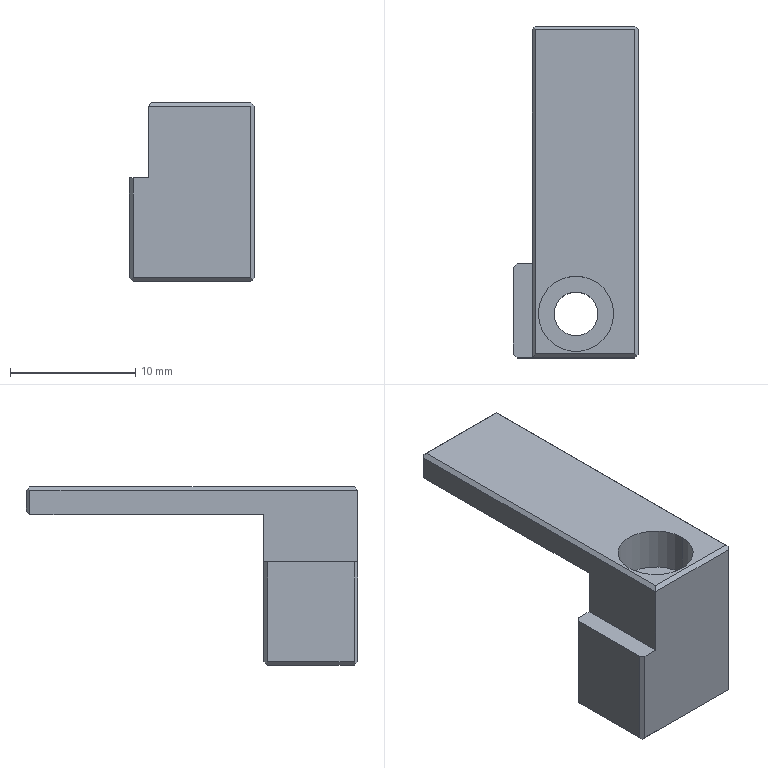Part | NX | 1 solid | 29 faces | box 10 x 26.45 x 14.25 mm | volume 1155 mm3 | plane 25 | cylinder 4 | commonest cylinder face diameters 3.5 x2 6 x2
STEP:
#1=CARTESIAN_POINT('',(-196.8,217.15,-49.35));
#2=VERTEX_POINT('',#1);
#3=CARTESIAN_POINT('',(-196.8,217.15,-47.4));
#4=VERTEX_POINT('',#3);
#5=CARTESIAN_POINT('',(-196.8,217.15,-48.375));
#6=DIRECTION('',(0.,0.,1.));
#7=VECTOR('',#6,1000.);
#8=LINE('',#5,#7);
#9=EDGE_CURVE('',#2,#4,#8,.T.);
#10=ORIENTED_EDGE('',*,*,#9,.T.);
#11=CARTESIAN_POINT('',(-196.8,191.3,-47.4));
#12=VERTEX_POINT('',#11);
#13=CARTESIAN_POINT('',(-196.8,212.,-47.4));
#14=DIRECTION('',(0.,-1.,0.));
#15=VECTOR('',#14,1000.);
#16=LINE('',#13,#15);
#17=EDGE_CURVE('',#4,#12,#16,.T.);
#18=ORIENTED_EDGE('',*,*,#17,.T.);
#19=CARTESIAN_POINT('',(-196.8,191.3,-61.05));
#20=VERTEX_POINT('',#19);
#21=CARTESIAN_POINT('',(-196.8,191.3,-54.225));
#22=DIRECTION('',(0.,0.,1.));
#23=VECTOR('',#22,1000.);
#24=LINE('',#21,#23);
#25=EDGE_CURVE('',#20,#12,#24,.T.);
#26=ORIENTED_EDGE('',*,*,#25,.F.);
#27=CARTESIAN_POINT('',(-196.8,198.5,-61.05));
#28=VERTEX_POINT('',#27);
#29=CARTESIAN_POINT('',(-196.8,194.75,-61.05));
#30=DIRECTION('',(0.,1.,0.));
#31=VECTOR('',#30,1000.);
#32=LINE('',#29,#31);
#33=EDGE_CURVE('',#20,#28,#32,.T.);
#34=ORIENTED_EDGE('',*,*,#33,.T.);
#35=CARTESIAN_POINT('',(-196.8,198.5,-49.35));
#36=VERTEX_POINT('',#35);
#37=CARTESIAN_POINT('',(-196.8,198.5,-40.731));
#38=DIRECTION('',(0.,0.,1.));
#39=VECTOR('',#38,1000.);
#40=LINE('',#37,#39);
#41=EDGE_CURVE('',#28,#36,#40,.T.);
#42=ORIENTED_EDGE('',*,*,#41,.T.);
#43=CARTESIAN_POINT('',(-196.8,212.,-49.35));
#44=DIRECTION('',(0.,-1.,0.));
#45=VECTOR('',#44,1000.);
#46=LINE('',#43,#45);
#47=EDGE_CURVE('',#2,#36,#46,.T.);
#48=ORIENTED_EDGE('',*,*,#47,.F.);
#49=EDGE_LOOP('',(#10,#18,#26,#34,#42,#48));
#50=FACE_BOUND('',#49,.T.);
#51=CARTESIAN_POINT('',(-196.8,212.,-46.1));
#52=DIRECTION('',(1.,0.,0.));
#53=DIRECTION('',(0.,1.,0.));
#54=AXIS2_PLACEMENT_3D('',#51,#52,#53);
#55=PLANE('',#54);
#56=ADVANCED_FACE('',(#50),#55,.T.);
#57=CARTESIAN_POINT('',(-197.1,217.15,-47.1));
#58=VERTEX_POINT('',#57);
#59=CARTESIAN_POINT('',(-205.,217.15,-47.1));
#60=VERTEX_POINT('',#59);
#61=CARTESIAN_POINT('',(-201.05,217.15,-47.1));
#62=DIRECTION('',(-1.,0.,0.));
#63=VECTOR('',#62,1000.);
#64=LINE('',#61,#63);
#65=EDGE_CURVE('',#58,#60,#64,.T.);
#66=ORIENTED_EDGE('',*,*,#65,.T.);
#67=CARTESIAN_POINT('',(-205.,191.3,-47.1));
#68=VERTEX_POINT('',#67);
#69=CARTESIAN_POINT('',(-205.,212.,-47.1));
#70=DIRECTION('',(0.,1.,0.));
#71=VECTOR('',#70,1000.);
#72=LINE('',#69,#71);
#73=EDGE_CURVE('',#68,#60,#72,.T.);
#74=ORIENTED_EDGE('',*,*,#73,.F.);
#75=CARTESIAN_POINT('',(-197.1,191.3,-47.1));
#76=VERTEX_POINT('',#75);
#77=CARTESIAN_POINT('',(-213.325,191.3,-47.1));
#78=DIRECTION('',(1.,0.,0.));
#79=VECTOR('',#78,1000.);
#80=LINE('',#77,#79);
#81=EDGE_CURVE('',#68,#76,#80,.T.);
#82=ORIENTED_EDGE('',*,*,#81,.T.);
#83=CARTESIAN_POINT('',(-197.1,212.,-47.1));
#84=DIRECTION('',(0.,-1.,0.));
#85=VECTOR('',#84,1000.);
#86=LINE('',#83,#85);
#87=EDGE_CURVE('',#58,#76,#86,.T.);
#88=ORIENTED_EDGE('',*,*,#87,.F.);
#89=EDGE_LOOP('',(#66,#74,#82,#88));
#90=FACE_BOUND('',#89,.T.);
#91=CARTESIAN_POINT('',(-198.8,194.5,-47.1));
#92=VERTEX_POINT('',#91);
#93=CARTESIAN_POINT('',(-204.8,194.5,-47.1));
#94=VERTEX_POINT('',#93);
#95=CARTESIAN_POINT('',(-201.8,194.5,-47.1));
#96=DIRECTION('',(0.,0.,1.));
#97=DIRECTION('',(-1.,0.,0.));
#98=AXIS2_PLACEMENT_3D('',#95,#96,#97);
#99=CIRCLE('',#98,3.);
#100=EDGE_CURVE('',#92,#94,#99,.T.);
#101=ORIENTED_EDGE('',*,*,#100,.F.);
#102=CARTESIAN_POINT('',(-201.8,194.5,-47.1));
#103=DIRECTION('',(0.,0.,1.));
#104=DIRECTION('',(-1.,0.,0.));
#105=AXIS2_PLACEMENT_3D('',#102,#103,#104);
#106=CIRCLE('',#105,3.);
#107=EDGE_CURVE('',#94,#92,#106,.T.);
#108=ORIENTED_EDGE('',*,*,#107,.F.);
#109=EDGE_LOOP('',(#101,#108));
#110=FACE_BOUND('',#109,.T.);
#111=CARTESIAN_POINT('',(-207.8,212.,-47.1));
#112=DIRECTION('',(0.,0.,1.));
#113=DIRECTION('',(0.,-1.,0.));
#114=AXIS2_PLACEMENT_3D('',#111,#112,#113);
#115=PLANE('',#114);
#116=ADVANCED_FACE('',(#90,#110),#115,.T.);
#117=CARTESIAN_POINT('',(-205.3,217.15,-49.35));
#118=VERTEX_POINT('',#117);
#119=CARTESIAN_POINT('',(-201.05,217.15,-49.35));
#120=DIRECTION('',(1.,0.,0.));
#121=VECTOR('',#120,1000.);
#122=LINE('',#119,#121);
#123=EDGE_CURVE('',#118,#2,#122,.T.);
#124=ORIENTED_EDGE('',*,*,#123,.T.);
#125=ORIENTED_EDGE('',*,*,#47,.T.);
#126=CARTESIAN_POINT('',(-205.3,198.5,-49.35));
#127=VERTEX_POINT('',#126);
#128=CARTESIAN_POINT('',(-213.325,198.5,-49.35));
#129=DIRECTION('',(1.,0.,0.));
#130=VECTOR('',#129,1000.);
#131=LINE('',#128,#130);
#132=EDGE_CURVE('',#127,#36,#131,.T.);
#133=ORIENTED_EDGE('',*,*,#132,.F.);
#134=CARTESIAN_POINT('',(-205.3,212.,-49.35));
#135=DIRECTION('',(0.,-1.,0.));
#136=VECTOR('',#135,1000.);
#137=LINE('',#134,#136);
#138=EDGE_CURVE('',#118,#127,#137,.T.);
#139=ORIENTED_EDGE('',*,*,#138,.F.);
#140=EDGE_LOOP('',(#124,#125,#133,#139));
#141=FACE_BOUND('',#140,.T.);
#142=CARTESIAN_POINT('',(-195.8,212.,-49.35));
#143=DIRECTION('',(0.,0.,-1.));
#144=DIRECTION('',(-1.,0.,0.));
#145=AXIS2_PLACEMENT_3D('',#142,#143,#144);
#146=PLANE('',#145);
#147=ADVANCED_FACE('',(#141),#146,.T.);
#148=CARTESIAN_POINT('',(-206.8,198.2,-53.1));
#149=VERTEX_POINT('',#148);
#150=CARTESIAN_POINT('',(-206.8,198.2,-61.05));
#151=VERTEX_POINT('',#150);
#152=CARTESIAN_POINT('',(-206.8,198.2,-57.225));
#153=DIRECTION('',(0.,0.,-1.));
#154=VECTOR('',#153,1000.);
#155=LINE('',#152,#154);
#156=EDGE_CURVE('',#149,#151,#155,.T.);
#157=ORIENTED_EDGE('',*,*,#156,.T.);
#158=CARTESIAN_POINT('',(-206.8,191.3,-61.05));
#159=VERTEX_POINT('',#158);
#160=CARTESIAN_POINT('',(-206.8,194.75,-61.05));
#161=DIRECTION('',(0.,-1.,0.));
#162=VECTOR('',#161,1000.);
#163=LINE('',#160,#162);
#164=EDGE_CURVE('',#151,#159,#163,.T.);
#165=ORIENTED_EDGE('',*,*,#164,.T.);
#166=CARTESIAN_POINT('',(-206.8,191.3,-53.1));
#167=VERTEX_POINT('',#166);
#168=CARTESIAN_POINT('',(-206.8,191.3,-57.225));
#169=DIRECTION('',(0.,0.,-1.));
#170=VECTOR('',#169,1000.);
#171=LINE('',#168,#170);
#172=EDGE_CURVE('',#167,#159,#171,.T.);
#173=ORIENTED_EDGE('',*,*,#172,.F.);
#174=CARTESIAN_POINT('',(-206.8,212.,-53.1));
#175=DIRECTION('',(0.,-1.,0.));
#176=VECTOR('',#175,1000.);
#177=LINE('',#174,#176);
#178=EDGE_CURVE('',#149,#167,#177,.T.);
#179=ORIENTED_EDGE('',*,*,#178,.F.);
#180=EDGE_LOOP('',(#157,#165,#173,#179));
#181=FACE_BOUND('',#180,.T.);
#182=CARTESIAN_POINT('',(-206.8,212.,-50.35));
#183=DIRECTION('',(-1.,0.,0.));
#184=DIRECTION('',(0.,1.,0.));
#185=AXIS2_PLACEMENT_3D('',#182,#183,#184);
#186=PLANE('',#185);
#187=ADVANCED_FACE('',(#181),#186,.T.);
#188=CARTESIAN_POINT('',(-197.1,191.3,-61.35));
#189=VERTEX_POINT('',#188);
#190=CARTESIAN_POINT('',(-197.1,198.2,-61.35));
#191=VERTEX_POINT('',#190);
#192=CARTESIAN_POINT('',(-197.1,194.75,-61.35));
#193=DIRECTION('',(0.,1.,0.));
#194=VECTOR('',#193,1000.);
#195=LINE('',#192,#194);
#196=EDGE_CURVE('',#189,#191,#195,.T.);
#197=ORIENTED_EDGE('',*,*,#196,.F.);
#198=CARTESIAN_POINT('',(-206.5,191.3,-61.35));
#199=VERTEX_POINT('',#198);
#200=CARTESIAN_POINT('',(-201.8,191.3,-61.35));
#201=DIRECTION('',(-1.,0.,0.));
#202=VECTOR('',#201,1000.);
#203=LINE('',#200,#202);
#204=EDGE_CURVE('',#189,#199,#203,.T.);
#205=ORIENTED_EDGE('',*,*,#204,.T.);
#206=CARTESIAN_POINT('',(-206.5,198.2,-61.35));
#207=VERTEX_POINT('',#206);
#208=CARTESIAN_POINT('',(-206.5,194.75,-61.35));
#209=DIRECTION('',(0.,-1.,0.));
#210=VECTOR('',#209,1000.);
#211=LINE('',#208,#210);
#212=EDGE_CURVE('',#207,#199,#211,.T.);
#213=ORIENTED_EDGE('',*,*,#212,.F.);
#214=CARTESIAN_POINT('',(-201.8,198.2,-61.35));
#215=DIRECTION('',(-1.,0.,0.));
#216=VECTOR('',#215,1000.);
#217=LINE('',#214,#216);
#218=EDGE_CURVE('',#191,#207,#217,.T.);
#219=ORIENTED_EDGE('',*,*,#218,.F.);
#220=EDGE_LOOP('',(#197,#205,#213,#219));
#221=FACE_BOUND('',#220,.T.);
#222=CARTESIAN_POINT('',(-200.05,194.5,-61.35));
#223=VERTEX_POINT('',#222);
#224=CARTESIAN_POINT('',(-203.55,194.5,-61.35));
#225=VERTEX_POINT('',#224);
#226=CARTESIAN_POINT('',(-201.8,194.5,-61.35));
#227=DIRECTION('',(0.,0.,1.));
#228=DIRECTION('',(-1.,0.,0.));
#229=AXIS2_PLACEMENT_3D('',#226,#227,#228);
#230=CIRCLE('',#229,1.75);
#231=EDGE_CURVE('',#223,#225,#230,.T.);
#232=ORIENTED_EDGE('',*,*,#231,.T.);
#233=CARTESIAN_POINT('',(-201.8,194.5,-61.35));
#234=DIRECTION('',(0.,0.,1.));
#235=DIRECTION('',(-1.,0.,0.));
#236=AXIS2_PLACEMENT_3D('',#233,#234,#235);
#237=CIRCLE('',#236,1.75);
#238=EDGE_CURVE('',#225,#223,#237,.T.);
#239=ORIENTED_EDGE('',*,*,#238,.T.);
#240=EDGE_LOOP('',(#232,#239));
#241=FACE_BOUND('',#240,.T.);
#242=CARTESIAN_POINT('',(-200.781,198.33,-61.35));
#243=DIRECTION('',(0.,0.,-1.));
#244=DIRECTION('',(-1.,0.,0.));
#245=AXIS2_PLACEMENT_3D('',#242,#243,#244);
#246=PLANE('',#245);
#247=ADVANCED_FACE('',(#221,#241),#246,.T.);
#248=ORIENTED_EDGE('',*,*,#100,.T.);
#249=CARTESIAN_POINT('',(-204.8,194.5,-50.6));
#250=VERTEX_POINT('',#249);
#251=CARTESIAN_POINT('',(-204.8,194.5,-47.1));
#252=DIRECTION('',(0.,0.,1.));
#253=VECTOR('',#252,1000.);
#254=LINE('',#251,#253);
#255=EDGE_CURVE('',#94,#250,#254,.F.);
#256=ORIENTED_EDGE('',*,*,#255,.T.);
#257=CARTESIAN_POINT('',(-198.8,194.5,-50.6));
#258=VERTEX_POINT('',#257);
#259=CARTESIAN_POINT('',(-201.8,194.5,-50.6));
#260=DIRECTION('',(0.,0.,1.));
#261=DIRECTION('',(-1.,0.,0.));
#262=AXIS2_PLACEMENT_3D('',#259,#260,#261);
#263=CIRCLE('',#262,3.);
#264=EDGE_CURVE('',#258,#250,#263,.T.);
#265=ORIENTED_EDGE('',*,*,#264,.F.);
#266=CARTESIAN_POINT('',(-198.8,194.5,-47.1));
#267=DIRECTION('',(0.,0.,1.));
#268=VECTOR('',#267,1000.);
#269=LINE('',#266,#268);
#270=EDGE_CURVE('',#92,#258,#269,.F.);
#271=ORIENTED_EDGE('',*,*,#270,.F.);
#272=EDGE_LOOP('',(#248,#256,#265,#271));
#273=FACE_BOUND('',#272,.T.);
#274=CARTESIAN_POINT('',(-201.8,194.5,-47.1));
#275=DIRECTION('',(0.,0.,1.));
#276=DIRECTION('',(-1.,0.,0.));
#277=AXIS2_PLACEMENT_3D('',#274,#275,#276);
#278=CYLINDRICAL_SURFACE('',#277,3.);
#279=ADVANCED_FACE('',(#273),#278,.F.);
#280=CARTESIAN_POINT('',(-200.05,194.5,-50.6));
#281=VERTEX_POINT('',#280);
#282=CARTESIAN_POINT('',(-203.55,194.5,-50.6));
#283=VERTEX_POINT('',#282);
#284=CARTESIAN_POINT('',(-201.8,194.5,-50.6));
#285=DIRECTION('',(0.,0.,1.));
#286=DIRECTION('',(-1.,0.,0.));
#287=AXIS2_PLACEMENT_3D('',#284,#285,#286);
#288=CIRCLE('',#287,1.75);
#289=EDGE_CURVE('',#281,#283,#288,.T.);
#290=ORIENTED_EDGE('',*,*,#289,.T.);
#291=CARTESIAN_POINT('',(-203.55,194.5,-47.1));
#292=DIRECTION('',(0.,0.,1.));
#293=VECTOR('',#292,1000.);
#294=LINE('',#291,#293);
#295=EDGE_CURVE('',#283,#225,#294,.F.);
#296=ORIENTED_EDGE('',*,*,#295,.T.);
#297=ORIENTED_EDGE('',*,*,#231,.F.);
#298=CARTESIAN_POINT('',(-200.05,194.5,-47.1));
#299=DIRECTION('',(0.,0.,1.));
#300=VECTOR('',#299,1000.);
#301=LINE('',#298,#300);
#302=EDGE_CURVE('',#281,#223,#301,.F.);
#303=ORIENTED_EDGE('',*,*,#302,.F.);
#304=EDGE_LOOP('',(#290,#296,#297,#303));
#305=FACE_BOUND('',#304,.T.);
#306=CARTESIAN_POINT('',(-201.8,194.5,-47.1));
#307=DIRECTION('',(0.,0.,1.));
#308=DIRECTION('',(-1.,0.,0.));
#309=AXIS2_PLACEMENT_3D('',#306,#307,#308);
#310=CYLINDRICAL_SURFACE('',#309,1.75);
#311=ADVANCED_FACE('',(#305),#310,.F.);
#312=ORIENTED_EDGE('',*,*,#264,.T.);
#313=CARTESIAN_POINT('',(-201.8,194.5,-50.6));
#314=DIRECTION('',(0.,0.,1.));
#315=DIRECTION('',(-1.,0.,0.));
#316=AXIS2_PLACEMENT_3D('',#313,#314,#315);
#317=CIRCLE('',#316,3.);
#318=EDGE_CURVE('',#250,#258,#317,.T.);
#319=ORIENTED_EDGE('',*,*,#318,.T.);
#320=EDGE_LOOP('',(#312,#319));
#321=FACE_BOUND('',#320,.T.);
#322=ORIENTED_EDGE('',*,*,#289,.F.);
#323=CARTESIAN_POINT('',(-201.8,194.5,-50.6));
#324=DIRECTION('',(0.,0.,1.));
#325=DIRECTION('',(-1.,0.,0.));
#326=AXIS2_PLACEMENT_3D('',#323,#324,#325);
#327=CIRCLE('',#326,1.75);
#328=EDGE_CURVE('',#283,#281,#327,.T.);
#329=ORIENTED_EDGE('',*,*,#328,.F.);
#330=EDGE_LOOP('',(#322,#329));
#331=FACE_BOUND('',#330,.T.);
#332=CARTESIAN_POINT('',(-201.8,194.5,-50.6));
#333=DIRECTION('',(0.,0.,1.));
#334=DIRECTION('',(0.,-1.,0.));
#335=AXIS2_PLACEMENT_3D('',#332,#333,#334);
#336=PLANE('',#335);
#337=ADVANCED_FACE('',(#321,#331),#336,.T.);
#338=CARTESIAN_POINT('',(-205.3,217.15,-47.4));
#339=VERTEX_POINT('',#338);
#340=CARTESIAN_POINT('',(-205.3,217.15,-48.375));
#341=DIRECTION('',(0.,0.,1.));
#342=VECTOR('',#341,1000.);
#343=LINE('',#340,#342);
#344=EDGE_CURVE('',#118,#339,#343,.T.);
#345=ORIENTED_EDGE('',*,*,#344,.F.);
#346=ORIENTED_EDGE('',*,*,#138,.T.);
#347=CARTESIAN_POINT('',(-205.3,198.5,-53.1));
#348=VERTEX_POINT('',#347);
#349=CARTESIAN_POINT('',(-205.3,198.5,-40.731));
#350=DIRECTION('',(0.,0.,-1.));
#351=VECTOR('',#350,1000.);
#352=LINE('',#349,#351);
#353=EDGE_CURVE('',#127,#348,#352,.T.);
#354=ORIENTED_EDGE('',*,*,#353,.T.);
#355=CARTESIAN_POINT('',(-205.3,191.,-53.1));
#356=VERTEX_POINT('',#355);
#357=CARTESIAN_POINT('',(-205.3,188.9,-53.1));
#358=DIRECTION('',(0.,1.,0.));
#359=VECTOR('',#358,1000.);
#360=LINE('',#357,#359);
#361=EDGE_CURVE('',#356,#348,#360,.T.);
#362=ORIENTED_EDGE('',*,*,#361,.F.);
#363=CARTESIAN_POINT('',(-205.3,191.,-47.4));
#364=VERTEX_POINT('',#363);
#365=CARTESIAN_POINT('',(-205.3,191.,-40.731));
#366=DIRECTION('',(0.,0.,-1.));
#367=VECTOR('',#366,1000.);
#368=LINE('',#365,#367);
#369=EDGE_CURVE('',#364,#356,#368,.T.);
#370=ORIENTED_EDGE('',*,*,#369,.F.);
#371=CARTESIAN_POINT('',(-205.3,212.,-47.4));
#372=DIRECTION('',(0.,1.,0.));
#373=VECTOR('',#372,1000.);
#374=LINE('',#371,#373);
#375=EDGE_CURVE('',#364,#339,#374,.T.);
#376=ORIENTED_EDGE('',*,*,#375,.T.);
#377=EDGE_LOOP('',(#345,#346,#354,#362,#370,#376));
#378=FACE_BOUND('',#377,.T.);
#379=CARTESIAN_POINT('',(-205.3,188.9,-53.1));
#380=DIRECTION('',(1.,0.,0.));
#381=DIRECTION('',(0.,1.,0.));
#382=AXIS2_PLACEMENT_3D('',#379,#380,#381);
#383=PLANE('',#382);
#384=ADVANCED_FACE('',(#378),#383,.F.);
#385=ORIENTED_EDGE('',*,*,#178,.T.);
#386=CARTESIAN_POINT('',(-206.5,191.,-53.1));
#387=VERTEX_POINT('',#386);
#388=CARTESIAN_POINT('',(-227.5,212.,-53.1));
#389=DIRECTION('',(0.7071,-0.7071,0.));
#390=VECTOR('',#389,1000.);
#391=LINE('',#388,#390);
#392=EDGE_CURVE('',#167,#387,#391,.T.);
#393=ORIENTED_EDGE('',*,*,#392,.T.);
#394=CARTESIAN_POINT('',(-213.325,191.,-53.1));
#395=DIRECTION('',(-1.,0.,0.));
#396=VECTOR('',#395,1000.);
#397=LINE('',#394,#396);
#398=EDGE_CURVE('',#356,#387,#397,.T.);
#399=ORIENTED_EDGE('',*,*,#398,.F.);
#400=ORIENTED_EDGE('',*,*,#361,.T.);
#401=CARTESIAN_POINT('',(-206.5,198.5,-53.1));
#402=VERTEX_POINT('',#401);
#403=CARTESIAN_POINT('',(-213.325,198.5,-53.1));
#404=DIRECTION('',(-1.,0.,0.));
#405=VECTOR('',#404,1000.);
#406=LINE('',#403,#405);
#407=EDGE_CURVE('',#348,#402,#406,.T.);
#408=ORIENTED_EDGE('',*,*,#407,.T.);
#409=CARTESIAN_POINT('',(-193.,212.,-53.1));
#410=DIRECTION('',(-0.7071,-0.7071,0.));
#411=VECTOR('',#410,1000.);
#412=LINE('',#409,#411);
#413=EDGE_CURVE('',#402,#149,#412,.T.);
#414=ORIENTED_EDGE('',*,*,#413,.T.);
#415=EDGE_LOOP('',(#385,#393,#399,#400,#408,#414));
#416=FACE_BOUND('',#415,.T.);
#417=CARTESIAN_POINT('',(-210.5,188.9,-53.1));
#418=DIRECTION('',(0.,0.,-1.));
#419=DIRECTION('',(-1.,0.,0.));
#420=AXIS2_PLACEMENT_3D('',#417,#418,#419);
#421=PLANE('',#420);
#422=ADVANCED_FACE('',(#416),#421,.F.);
#423=ORIENTED_EDGE('',*,*,#218,.T.);
#424=CARTESIAN_POINT('',(-206.65,198.35,-61.2));
#425=VERTEX_POINT('',#424);
#426=CARTESIAN_POINT('',(-220.3,212.,-47.55));
#427=DIRECTION('',(0.5774,-0.5774,-0.5774));
#428=VECTOR('',#427,1000.);
#429=LINE('',#426,#428);
#430=EDGE_CURVE('',#425,#207,#429,.T.);
#431=ORIENTED_EDGE('',*,*,#430,.F.);
#432=CARTESIAN_POINT('',(-206.5,198.5,-61.05));
#433=VERTEX_POINT('',#432);
#434=CARTESIAN_POINT('',(-186.181,218.819,-40.731));
#435=DIRECTION('',(-0.5774,-0.5774,-0.5774));
#436=VECTOR('',#435,1000.);
#437=LINE('',#434,#436);
#438=EDGE_CURVE('',#433,#425,#437,.T.);
#439=ORIENTED_EDGE('',*,*,#438,.F.);
#440=CARTESIAN_POINT('',(-201.8,198.5,-61.05));
#441=DIRECTION('',(-1.,0.,0.));
#442=VECTOR('',#441,1000.);
#443=LINE('',#440,#442);
#444=EDGE_CURVE('',#28,#433,#443,.T.);
#445=ORIENTED_EDGE('',*,*,#444,.F.);
#446=CARTESIAN_POINT('',(-183.3,212.,-47.55));
#447=DIRECTION('',(-0.5774,-0.5774,-0.5774));
#448=VECTOR('',#447,1000.);
#449=LINE('',#446,#448);
#450=EDGE_CURVE('',#28,#191,#449,.T.);
#451=ORIENTED_EDGE('',*,*,#450,.T.);
#452=EDGE_LOOP('',(#423,#431,#439,#445,#451));
#453=FACE_BOUND('',#452,.T.);
#454=CARTESIAN_POINT('',(-201.8,198.35,-61.2));
#455=DIRECTION('',(0.,-0.7071,0.7071));
#456=DIRECTION('',(-1.,0.,0.));
#457=AXIS2_PLACEMENT_3D('',#454,#455,#456);
#458=PLANE('',#457);
#459=ADVANCED_FACE('',(#453),#458,.F.);
#460=ORIENTED_EDGE('',*,*,#156,.F.);
#461=ORIENTED_EDGE('',*,*,#413,.F.);
#462=CARTESIAN_POINT('',(-206.5,198.5,-57.225));
#463=DIRECTION('',(0.,0.,-1.));
#464=VECTOR('',#463,1000.);
#465=LINE('',#462,#464);
#466=EDGE_CURVE('',#402,#433,#465,.T.);
#467=ORIENTED_EDGE('',*,*,#466,.T.);
#468=ORIENTED_EDGE('',*,*,#438,.T.);
#469=CARTESIAN_POINT('',(-193.,212.,-74.85));
#470=DIRECTION('',(-0.5774,-0.5774,0.5774));
#471=VECTOR('',#470,1000.);
#472=LINE('',#469,#471);
#473=EDGE_CURVE('',#425,#151,#472,.T.);
#474=ORIENTED_EDGE('',*,*,#473,.T.);
#475=EDGE_LOOP('',(#460,#461,#467,#468,#474));
#476=FACE_BOUND('',#475,.T.);
#477=CARTESIAN_POINT('',(-206.65,198.35,-57.225));
#478=DIRECTION('',(-0.7071,0.7071,0.));
#479=DIRECTION('',(0.,0.,1.));
#480=AXIS2_PLACEMENT_3D('',#477,#478,#479);
#481=PLANE('',#480);
#482=ADVANCED_FACE('',(#476),#481,.T.);
#483=ORIENTED_EDGE('',*,*,#196,.T.);
#484=ORIENTED_EDGE('',*,*,#450,.F.);
#485=ORIENTED_EDGE('',*,*,#33,.F.);
#486=CARTESIAN_POINT('',(-196.95,191.15,-61.2));
#487=VERTEX_POINT('',#486);
#488=CARTESIAN_POINT('',(-176.1,212.,-40.35));
#489=DIRECTION('',(-0.5774,-0.5774,-0.5774));
#490=VECTOR('',#489,1000.);
#491=LINE('',#488,#490);
#492=EDGE_CURVE('',#20,#487,#491,.T.);
#493=ORIENTED_EDGE('',*,*,#492,.T.);
#494=CARTESIAN_POINT('',(-217.8,212.,-82.05));
#495=DIRECTION('',(-0.5774,0.5774,-0.5774));
#496=VECTOR('',#495,1000.);
#497=LINE('',#494,#496);
#498=EDGE_CURVE('',#487,#189,#497,.T.);
#499=ORIENTED_EDGE('',*,*,#498,.T.);
#500=EDGE_LOOP('',(#483,#484,#485,#493,#499));
#501=FACE_BOUND('',#500,.T.);
#502=CARTESIAN_POINT('',(-196.95,194.75,-61.2));
#503=DIRECTION('',(-0.7071,0.,0.7071));
#504=DIRECTION('',(0.,1.,0.));
#505=AXIS2_PLACEMENT_3D('',#502,#503,#504);
#506=PLANE('',#505);
#507=ADVANCED_FACE('',(#501),#506,.F.);
#508=ORIENTED_EDGE('',*,*,#204,.F.);
#509=ORIENTED_EDGE('',*,*,#498,.F.);
#510=CARTESIAN_POINT('',(-197.1,191.,-61.05));
#511=VERTEX_POINT('',#510);
#512=CARTESIAN_POINT('',(-176.1,212.,-82.05));
#513=DIRECTION('',(0.5774,0.5774,-0.5774));
#514=VECTOR('',#513,1000.);
#515=LINE('',#512,#514);
#516=EDGE_CURVE('',#511,#487,#515,.T.);
#517=ORIENTED_EDGE('',*,*,#516,.F.);
#518=CARTESIAN_POINT('',(-206.5,191.,-61.05));
#519=VERTEX_POINT('',#518);
#520=CARTESIAN_POINT('',(-201.8,191.,-61.05));
#521=DIRECTION('',(-1.,0.,0.));
#522=VECTOR('',#521,1000.);
#523=LINE('',#520,#522);
#524=EDGE_CURVE('',#511,#519,#523,.T.);
#525=ORIENTED_EDGE('',*,*,#524,.T.);
#526=CARTESIAN_POINT('',(-206.65,191.15,-61.2));
#527=VERTEX_POINT('',#526);
#528=CARTESIAN_POINT('',(-227.5,212.,-82.05));
#529=DIRECTION('',(0.5774,-0.5774,0.5774));
#530=VECTOR('',#529,1000.);
#531=LINE('',#528,#530);
#532=EDGE_CURVE('',#527,#519,#531,.T.);
#533=ORIENTED_EDGE('',*,*,#532,.F.);
#534=CARTESIAN_POINT('',(-185.8,212.,-82.05));
#535=DIRECTION('',(-0.5774,-0.5774,0.5774));
#536=VECTOR('',#535,1000.);
#537=LINE('',#534,#536);
#538=EDGE_CURVE('',#199,#527,#537,.T.);
#539=ORIENTED_EDGE('',*,*,#538,.F.);
#540=EDGE_LOOP('',(#508,#509,#517,#525,#533,#539));
#541=FACE_BOUND('',#540,.T.);
#542=CARTESIAN_POINT('',(-201.8,191.15,-61.2));
#543=DIRECTION('',(0.,-0.7071,-0.7071));
#544=DIRECTION('',(0.,-0.7071,0.7071));
#545=AXIS2_PLACEMENT_3D('',#542,#543,#544);
#546=PLANE('',#545);
#547=ADVANCED_FACE('',(#541),#546,.T.);
#548=ORIENTED_EDGE('',*,*,#212,.T.);
#549=ORIENTED_EDGE('',*,*,#538,.T.);
#550=CARTESIAN_POINT('',(-227.5,212.,-40.35));
#551=DIRECTION('',(-0.5774,0.5774,0.5774));
#552=VECTOR('',#551,1000.);
#553=LINE('',#550,#552);
#554=EDGE_CURVE('',#527,#159,#553,.T.);
#555=ORIENTED_EDGE('',*,*,#554,.T.);
#556=ORIENTED_EDGE('',*,*,#164,.F.);
#557=ORIENTED_EDGE('',*,*,#473,.F.);
#558=ORIENTED_EDGE('',*,*,#430,.T.);
#559=EDGE_LOOP('',(#548,#549,#555,#556,#557,#558));
#560=FACE_BOUND('',#559,.T.);
#561=CARTESIAN_POINT('',(-206.65,194.75,-61.2));
#562=DIRECTION('',(0.7071,0.,0.7071));
#563=DIRECTION('',(0.,-1.,0.));
#564=AXIS2_PLACEMENT_3D('',#561,#562,#563);
#565=PLANE('',#564);
#566=ADVANCED_FACE('',(#560),#565,.F.);
#567=ORIENTED_EDGE('',*,*,#17,.F.);
#568=CARTESIAN_POINT('',(-196.95,217.3,-47.25));
#569=VERTEX_POINT('',#568);
#570=CARTESIAN_POINT('',(-213.325,233.675,-30.875));
#571=DIRECTION('',(0.5774,-0.5774,-0.5774));
#572=VECTOR('',#571,1000.);
#573=LINE('',#570,#572);
#574=EDGE_CURVE('',#569,#4,#573,.T.);
#575=ORIENTED_EDGE('',*,*,#574,.F.);
#576=CARTESIAN_POINT('',(-213.325,200.925,-30.875));
#577=DIRECTION('',(0.5774,0.5774,-0.5774));
#578=VECTOR('',#577,1000.);
#579=LINE('',#576,#578);
#580=EDGE_CURVE('',#58,#569,#579,.T.);
#581=ORIENTED_EDGE('',*,*,#580,.F.);
#582=ORIENTED_EDGE('',*,*,#87,.T.);
#583=CARTESIAN_POINT('',(-196.95,191.15,-47.25));
#584=VERTEX_POINT('',#583);
#585=CARTESIAN_POINT('',(-217.8,212.,-26.4));
#586=DIRECTION('',(-0.5774,0.5774,0.5774));
#587=VECTOR('',#586,1000.);
#588=LINE('',#585,#587);
#589=EDGE_CURVE('',#584,#76,#588,.T.);
#590=ORIENTED_EDGE('',*,*,#589,.F.);
#591=CARTESIAN_POINT('',(-176.1,212.,-68.1));
#592=DIRECTION('',(0.5774,0.5774,-0.5774));
#593=VECTOR('',#592,1000.);
#594=LINE('',#591,#593);
#595=EDGE_CURVE('',#584,#12,#594,.T.);
#596=ORIENTED_EDGE('',*,*,#595,.T.);
#597=EDGE_LOOP('',(#567,#575,#581,#582,#590,#596));
#598=FACE_BOUND('',#597,.T.);
#599=CARTESIAN_POINT('',(-196.95,200.775,-47.25));
#600=DIRECTION('',(0.7071,0.,0.7071));
#601=DIRECTION('',(0.,-1.,0.));
#602=AXIS2_PLACEMENT_3D('',#599,#600,#601);
#603=PLANE('',#602);
#604=ADVANCED_FACE('',(#598),#603,.T.);
#605=ORIENTED_EDGE('',*,*,#375,.F.);
#606=CARTESIAN_POINT('',(-184.3,212.,-26.4));
#607=DIRECTION('',(0.5774,0.5774,0.5774));
#608=VECTOR('',#607,1000.);
#609=LINE('',#606,#608);
#610=EDGE_CURVE('',#364,#68,#609,.T.);
#611=ORIENTED_EDGE('',*,*,#610,.T.);
#612=ORIENTED_EDGE('',*,*,#73,.T.);
#613=CARTESIAN_POINT('',(-205.15,217.3,-47.25));
#614=VERTEX_POINT('',#613);
#615=CARTESIAN_POINT('',(-213.325,225.475,-55.425));
#616=DIRECTION('',(-0.5774,0.5774,-0.5774));
#617=VECTOR('',#616,1000.);
#618=LINE('',#615,#617);
#619=EDGE_CURVE('',#60,#614,#618,.T.);
#620=ORIENTED_EDGE('',*,*,#619,.T.);
#621=CARTESIAN_POINT('',(-210.45,212.,-52.55));
#622=DIRECTION('',(0.5774,0.5774,0.5774));
#623=VECTOR('',#622,1000.);
#624=LINE('',#621,#623);
#625=EDGE_CURVE('',#339,#614,#624,.T.);
#626=ORIENTED_EDGE('',*,*,#625,.F.);
#627=EDGE_LOOP('',(#605,#611,#612,#620,#626));
#628=FACE_BOUND('',#627,.T.);
#629=CARTESIAN_POINT('',(-205.15,200.775,-47.25));
#630=DIRECTION('',(0.7071,0.,-0.7071));
#631=DIRECTION('',(0.,-1.,0.));
#632=AXIS2_PLACEMENT_3D('',#629,#630,#631);
#633=PLANE('',#632);
#634=ADVANCED_FACE('',(#628),#633,.F.);
#635=ORIENTED_EDGE('',*,*,#65,.F.);
#636=ORIENTED_EDGE('',*,*,#580,.T.);
#637=CARTESIAN_POINT('',(-197.1,217.45,-47.4));
#638=VERTEX_POINT('',#637);
#639=CARTESIAN_POINT('',(-213.325,233.675,-63.625));
#640=DIRECTION('',(0.5774,-0.5774,0.5774));
#641=VECTOR('',#640,1000.);
#642=LINE('',#639,#641);
#643=EDGE_CURVE('',#638,#569,#642,.T.);
#644=ORIENTED_EDGE('',*,*,#643,.F.);
#645=CARTESIAN_POINT('',(-205.,217.45,-47.4));
#646=VERTEX_POINT('',#645);
#647=CARTESIAN_POINT('',(-201.05,217.45,-47.4));
#648=DIRECTION('',(-1.,0.,0.));
#649=VECTOR('',#648,1000.);
#650=LINE('',#647,#649);
#651=EDGE_CURVE('',#638,#646,#650,.T.);
#652=ORIENTED_EDGE('',*,*,#651,.T.);
#653=CARTESIAN_POINT('',(-210.45,212.,-41.95));
#654=DIRECTION('',(-0.5774,-0.5774,0.5774));
#655=VECTOR('',#654,1000.);
#656=LINE('',#653,#655);
#657=EDGE_CURVE('',#646,#614,#656,.T.);
#658=ORIENTED_EDGE('',*,*,#657,.T.);
#659=ORIENTED_EDGE('',*,*,#619,.F.);
#660=EDGE_LOOP('',(#635,#636,#644,#652,#658,#659));
#661=FACE_BOUND('',#660,.T.);
#662=CARTESIAN_POINT('',(-201.05,217.3,-47.25));
#663=DIRECTION('',(0.,0.7071,0.7071));
#664=DIRECTION('',(1.,0.,0.));
#665=AXIS2_PLACEMENT_3D('',#662,#663,#664);
#666=PLANE('',#665);
#667=ADVANCED_FACE('',(#661),#666,.T.);
#668=ORIENTED_EDGE('',*,*,#9,.F.);
#669=CARTESIAN_POINT('',(-197.1,217.45,-49.05));
#670=VERTEX_POINT('',#669);
#671=CARTESIAN_POINT('',(-205.419,225.769,-40.731));
#672=DIRECTION('',(0.5774,-0.5774,-0.5774));
#673=VECTOR('',#672,1000.);
#674=LINE('',#671,#673);
#675=EDGE_CURVE('',#670,#2,#674,.T.);
#676=ORIENTED_EDGE('',*,*,#675,.F.);
#677=CARTESIAN_POINT('',(-197.1,217.45,-48.375));
#678=DIRECTION('',(0.,0.,1.));
#679=VECTOR('',#678,1000.);
#680=LINE('',#677,#679);
#681=EDGE_CURVE('',#670,#638,#680,.T.);
#682=ORIENTED_EDGE('',*,*,#681,.T.);
#683=ORIENTED_EDGE('',*,*,#643,.T.);
#684=ORIENTED_EDGE('',*,*,#574,.T.);
#685=EDGE_LOOP('',(#668,#676,#682,#683,#684));
#686=FACE_BOUND('',#685,.T.);
#687=CARTESIAN_POINT('',(-196.95,217.3,-48.375));
#688=DIRECTION('',(0.7071,0.7071,0.));
#689=DIRECTION('',(0.,0.,-1.));
#690=AXIS2_PLACEMENT_3D('',#687,#688,#689);
#691=PLANE('',#690);
#692=ADVANCED_FACE('',(#686),#691,.T.);
#693=ORIENTED_EDGE('',*,*,#344,.T.);
#694=ORIENTED_EDGE('',*,*,#625,.T.);
#695=ORIENTED_EDGE('',*,*,#657,.F.);
#696=CARTESIAN_POINT('',(-205.,217.45,-49.05));
#697=VERTEX_POINT('',#696);
#698=CARTESIAN_POINT('',(-205.,217.45,-48.375));
#699=DIRECTION('',(0.,0.,1.));
#700=VECTOR('',#699,1000.);
#701=LINE('',#698,#700);
#702=EDGE_CURVE('',#697,#646,#701,.T.);
#703=ORIENTED_EDGE('',*,*,#702,.F.);
#704=CARTESIAN_POINT('',(-196.681,225.769,-40.731));
#705=DIRECTION('',(0.5774,0.5774,0.5774));
#706=VECTOR('',#705,1000.);
#707=LINE('',#704,#706);
#708=EDGE_CURVE('',#118,#697,#707,.T.);
#709=ORIENTED_EDGE('',*,*,#708,.F.);
#710=EDGE_LOOP('',(#693,#694,#695,#703,#709));
#711=FACE_BOUND('',#710,.T.);
#712=CARTESIAN_POINT('',(-205.15,217.3,-48.375));
#713=DIRECTION('',(0.7071,-0.7071,0.));
#714=DIRECTION('',(0.,0.,-1.));
#715=AXIS2_PLACEMENT_3D('',#712,#713,#714);
#716=PLANE('',#715);
#717=ADVANCED_FACE('',(#711),#716,.F.);
#718=ORIENTED_EDGE('',*,*,#255,.F.);
#719=ORIENTED_EDGE('',*,*,#107,.T.);
#720=ORIENTED_EDGE('',*,*,#270,.T.);
#721=ORIENTED_EDGE('',*,*,#318,.F.);
#722=EDGE_LOOP('',(#718,#719,#720,#721));
#723=FACE_BOUND('',#722,.T.);
#724=CARTESIAN_POINT('',(-201.8,194.5,-47.1));
#725=DIRECTION('',(0.,0.,1.));
#726=DIRECTION('',(-1.,0.,0.));
#727=AXIS2_PLACEMENT_3D('',#724,#725,#726);
#728=CYLINDRICAL_SURFACE('',#727,3.);
#729=ADVANCED_FACE('',(#723),#728,.F.);
#730=ORIENTED_EDGE('',*,*,#295,.F.);
#731=ORIENTED_EDGE('',*,*,#328,.T.);
#732=ORIENTED_EDGE('',*,*,#302,.T.);
#733=ORIENTED_EDGE('',*,*,#238,.F.);
#734=EDGE_LOOP('',(#730,#731,#732,#733));
#735=FACE_BOUND('',#734,.T.);
#736=CARTESIAN_POINT('',(-201.8,194.5,-47.1));
#737=DIRECTION('',(0.,0.,1.));
#738=DIRECTION('',(-1.,0.,0.));
#739=AXIS2_PLACEMENT_3D('',#736,#737,#738);
#740=CYLINDRICAL_SURFACE('',#739,1.75);
#741=ADVANCED_FACE('',(#735),#740,.F.);
#742=CARTESIAN_POINT('',(-206.5,191.,-57.225));
#743=DIRECTION('',(0.,0.,-1.));
#744=VECTOR('',#743,1000.);
#745=LINE('',#742,#744);
#746=EDGE_CURVE('',#387,#519,#745,.T.);
#747=ORIENTED_EDGE('',*,*,#746,.T.);
#748=ORIENTED_EDGE('',*,*,#524,.F.);
#749=CARTESIAN_POINT('',(-197.1,191.,-47.4));
#750=VERTEX_POINT('',#749);
#751=CARTESIAN_POINT('',(-197.1,191.,-54.225));
#752=DIRECTION('',(0.,0.,1.));
#753=VECTOR('',#752,1000.);
#754=LINE('',#751,#753);
#755=EDGE_CURVE('',#511,#750,#754,.T.);
#756=ORIENTED_EDGE('',*,*,#755,.T.);
#757=CARTESIAN_POINT('',(-201.05,191.,-47.4));
#758=DIRECTION('',(1.,0.,0.));
#759=VECTOR('',#758,1000.);
#760=LINE('',#757,#759);
#761=EDGE_CURVE('',#364,#750,#760,.T.);
#762=ORIENTED_EDGE('',*,*,#761,.F.);
#763=ORIENTED_EDGE('',*,*,#369,.T.);
#764=ORIENTED_EDGE('',*,*,#398,.T.);
#765=EDGE_LOOP('',(#747,#748,#756,#762,#763,#764));
#766=FACE_BOUND('',#765,.T.);
#767=CARTESIAN_POINT('',(-213.325,191.,-40.731));
#768=DIRECTION('',(0.,1.,0.));
#769=DIRECTION('',(0.,0.,-1.));
#770=AXIS2_PLACEMENT_3D('',#767,#768,#769);
#771=PLANE('',#770);
#772=ADVANCED_FACE('',(#766),#771,.F.);
#773=ORIENTED_EDGE('',*,*,#610,.F.);
#774=ORIENTED_EDGE('',*,*,#761,.T.);
#775=CARTESIAN_POINT('',(-176.1,212.,-26.4));
#776=DIRECTION('',(-0.5774,-0.5774,-0.5774));
#777=VECTOR('',#776,1000.);
#778=LINE('',#775,#777);
#779=EDGE_CURVE('',#584,#750,#778,.T.);
#780=ORIENTED_EDGE('',*,*,#779,.F.);
#781=ORIENTED_EDGE('',*,*,#589,.T.);
#782=ORIENTED_EDGE('',*,*,#81,.F.);
#783=EDGE_LOOP('',(#773,#774,#780,#781,#782));
#784=FACE_BOUND('',#783,.T.);
#785=CARTESIAN_POINT('',(-201.05,191.15,-47.25));
#786=DIRECTION('',(0.,0.7071,-0.7071));
#787=DIRECTION('',(-1.,0.,0.));
#788=AXIS2_PLACEMENT_3D('',#785,#786,#787);
#789=PLANE('',#788);
#790=ADVANCED_FACE('',(#784),#789,.F.);
#791=ORIENTED_EDGE('',*,*,#755,.F.);
#792=ORIENTED_EDGE('',*,*,#516,.T.);
#793=ORIENTED_EDGE('',*,*,#492,.F.);
#794=ORIENTED_EDGE('',*,*,#25,.T.);
#795=ORIENTED_EDGE('',*,*,#595,.F.);
#796=ORIENTED_EDGE('',*,*,#779,.T.);
#797=EDGE_LOOP('',(#791,#792,#793,#794,#795,#796));
#798=FACE_BOUND('',#797,.T.);
#799=CARTESIAN_POINT('',(-196.95,191.15,-54.225));
#800=DIRECTION('',(0.7071,-0.7071,0.));
#801=DIRECTION('',(0.,0.,-1.));
#802=AXIS2_PLACEMENT_3D('',#799,#800,#801);
#803=PLANE('',#802);
#804=ADVANCED_FACE('',(#798),#803,.T.);
#805=ORIENTED_EDGE('',*,*,#746,.F.);
#806=ORIENTED_EDGE('',*,*,#392,.F.);
#807=ORIENTED_EDGE('',*,*,#172,.T.);
#808=ORIENTED_EDGE('',*,*,#554,.F.);
#809=ORIENTED_EDGE('',*,*,#532,.T.);
#810=EDGE_LOOP('',(#805,#806,#807,#808,#809));
#811=FACE_BOUND('',#810,.T.);
#812=CARTESIAN_POINT('',(-206.65,191.15,-57.225));
#813=DIRECTION('',(-0.7071,-0.7071,0.));
#814=DIRECTION('',(-0.7071,0.7071,0.));
#815=AXIS2_PLACEMENT_3D('',#812,#813,#814);
#816=PLANE('',#815);
#817=ADVANCED_FACE('',(#811),#816,.T.);
#818=CARTESIAN_POINT('',(-201.05,217.45,-49.05));
#819=DIRECTION('',(1.,0.,0.));
#820=VECTOR('',#819,1000.);
#821=LINE('',#818,#820);
#822=EDGE_CURVE('',#697,#670,#821,.T.);
#823=ORIENTED_EDGE('',*,*,#822,.F.);
#824=ORIENTED_EDGE('',*,*,#702,.T.);
#825=ORIENTED_EDGE('',*,*,#651,.F.);
#826=ORIENTED_EDGE('',*,*,#681,.F.);
#827=EDGE_LOOP('',(#823,#824,#825,#826));
#828=FACE_BOUND('',#827,.T.);
#829=CARTESIAN_POINT('',(-213.325,217.45,-40.731));
#830=DIRECTION('',(0.,1.,0.));
#831=DIRECTION('',(0.,0.,-1.));
#832=AXIS2_PLACEMENT_3D('',#829,#830,#831);
#833=PLANE('',#832);
#834=ADVANCED_FACE('',(#828),#833,.T.);
#835=ORIENTED_EDGE('',*,*,#132,.T.);
#836=ORIENTED_EDGE('',*,*,#41,.F.);
#837=ORIENTED_EDGE('',*,*,#444,.T.);
#838=ORIENTED_EDGE('',*,*,#466,.F.);
#839=ORIENTED_EDGE('',*,*,#407,.F.);
#840=ORIENTED_EDGE('',*,*,#353,.F.);
#841=EDGE_LOOP('',(#835,#836,#837,#838,#839,#840));
#842=FACE_BOUND('',#841,.T.);
#843=CARTESIAN_POINT('',(-196.8,198.5,-49.35));
#844=DIRECTION('',(0.,1.,0.));
#845=DIRECTION('',(0.,0.,-1.));
#846=AXIS2_PLACEMENT_3D('',#843,#844,#845);
#847=PLANE('',#846);
#848=ADVANCED_FACE('',(#842),#847,.T.);
#849=ORIENTED_EDGE('',*,*,#822,.T.);
#850=ORIENTED_EDGE('',*,*,#675,.T.);
#851=ORIENTED_EDGE('',*,*,#123,.F.);
#852=ORIENTED_EDGE('',*,*,#708,.T.);
#853=EDGE_LOOP('',(#849,#850,#851,#852));
#854=FACE_BOUND('',#853,.T.);
#855=CARTESIAN_POINT('',(-201.05,217.3,-49.2));
#856=DIRECTION('',(0.,-0.7071,0.7071));
#857=DIRECTION('',(-1.,0.,0.));
#858=AXIS2_PLACEMENT_3D('',#855,#856,#857);
#859=PLANE('',#858);
#860=ADVANCED_FACE('',(#854),#859,.F.);
#861=CLOSED_SHELL('',(#56,#116,#147,#187,#247,#279,#311,#337,#384,#422,#459,#482,#507,#547,#566,#604,#634,#667,#692,#717,#729,#741,#772,#790,#804,#817,#834,#848,#860));
#862=MANIFOLD_SOLID_BREP('',#861);
#863=(LENGTH_UNIT()NAMED_UNIT(*)SI_UNIT(.MILLI.,.METRE.));
#864=UNCERTAINTY_MEASURE_WITH_UNIT(LENGTH_MEASURE(0.00001),#863,'','');
#865=(NAMED_UNIT(*)PLANE_ANGLE_UNIT()SI_UNIT($,.RADIAN.));
#866=(NAMED_UNIT(*)SI_UNIT($,.STERADIAN.)SOLID_ANGLE_UNIT());
#867=(GEOMETRIC_REPRESENTATION_CONTEXT(3)GLOBAL_UNCERTAINTY_ASSIGNED_CONTEXT((#864))GLOBAL_UNIT_ASSIGNED_CONTEXT((#863,#865,#866))REPRESENTATION_CONTEXT('',''));
#868=ADVANCED_BREP_SHAPE_REPRESENTATION('',(#862),#867);